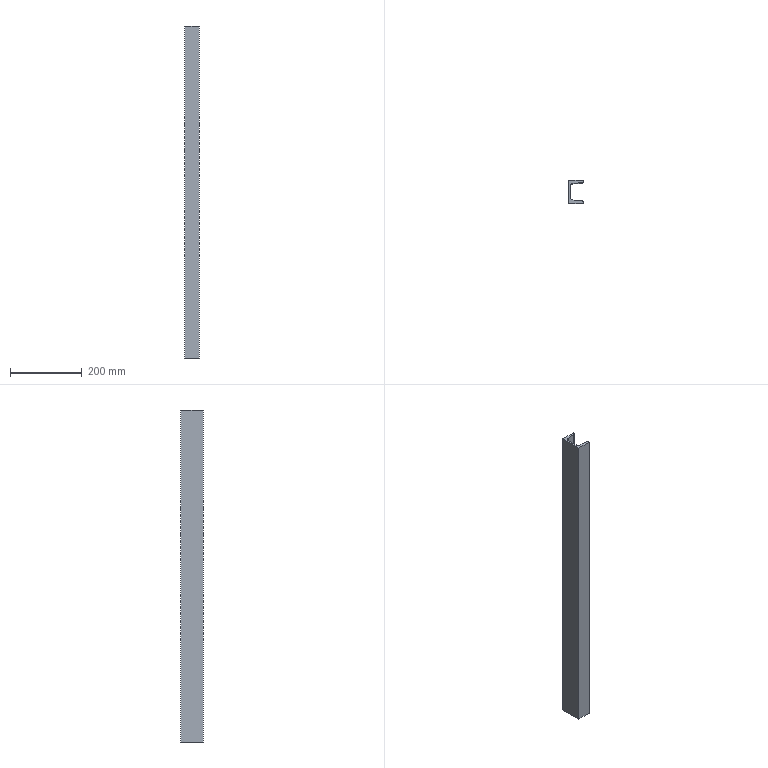Part | STEP file | 750038453 | 1 solid | 14 faces | box 40 x 63 x 924 mm | volume 780380 mm3 | plane 10 | cylinder 4 | commonest cylinder face diameters 7.6 x2 15 x2
STEP:
#1=CARTESIAN_POINT('',(0.,0.,462.));
#2=VERTEX_POINT('',#1);
#3=CARTESIAN_POINT('',(0.,0.,-462.));
#4=VERTEX_POINT('',#3);
#5=CARTESIAN_POINT('',(0.,0.,462.));
#6=DIRECTION('',(0.,0.,-1.));
#7=VECTOR('',#6,1000.);
#8=LINE('',#5,#7);
#9=EDGE_CURVE('',#2,#4,#8,.T.);
#10=ORIENTED_EDGE('',*,*,#9,.F.);
#11=CARTESIAN_POINT('',(0.,63.,462.));
#12=VERTEX_POINT('',#11);
#13=CARTESIAN_POINT('',(0.,63.,462.));
#14=DIRECTION('',(0.,-1.,0.));
#15=VECTOR('',#14,1000.);
#16=LINE('',#13,#15);
#17=EDGE_CURVE('',#12,#2,#16,.T.);
#18=ORIENTED_EDGE('',*,*,#17,.F.);
#19=CARTESIAN_POINT('',(0.,63.,-462.));
#20=VERTEX_POINT('',#19);
#21=CARTESIAN_POINT('',(0.,63.,462.));
#22=DIRECTION('',(0.,0.,1.));
#23=VECTOR('',#22,1000.);
#24=LINE('',#21,#23);
#25=EDGE_CURVE('',#20,#12,#24,.T.);
#26=ORIENTED_EDGE('',*,*,#25,.F.);
#27=CARTESIAN_POINT('',(0.,63.,-462.));
#28=DIRECTION('',(0.,1.,0.));
#29=VECTOR('',#28,1000.);
#30=LINE('',#27,#29);
#31=EDGE_CURVE('',#4,#20,#30,.T.);
#32=ORIENTED_EDGE('',*,*,#31,.F.);
#33=EDGE_LOOP('',(#10,#18,#26,#32));
#34=FACE_OUTER_BOUND('',#33,.T.);
#35=CARTESIAN_POINT('',(0.,63.,462.));
#36=DIRECTION('',(1.,0.,0.));
#37=DIRECTION('',(0.,0.,-1.));
#38=AXIS2_PLACEMENT_3D('',#35,#36,#37);
#39=PLANE('',#38);
#40=ADVANCED_FACE('',(#34),#39,.F.);
#41=CARTESIAN_POINT('',(40.,63.,-462.));
#42=VERTEX_POINT('',#41);
#43=CARTESIAN_POINT('',(36.2,63.,-462.));
#44=DIRECTION('',(-1.,0.,0.));
#45=VECTOR('',#44,1000.);
#46=LINE('',#43,#45);
#47=EDGE_CURVE('',#42,#20,#46,.T.);
#48=ORIENTED_EDGE('',*,*,#47,.F.);
#49=CARTESIAN_POINT('',(40.,60.699,-462.));
#50=VERTEX_POINT('',#49);
#51=CARTESIAN_POINT('',(40.,2.301,-462.));
#52=DIRECTION('',(0.,1.,0.));
#53=VECTOR('',#52,1000.);
#54=LINE('',#51,#53);
#55=EDGE_CURVE('',#50,#42,#54,.T.);
#56=ORIENTED_EDGE('',*,*,#55,.F.);
#57=CARTESIAN_POINT('',(36.578,56.918,-462.));
#58=VERTEX_POINT('',#57);
#59=CARTESIAN_POINT('',(36.2,60.699,-462.));
#60=DIRECTION('',(0.,0.,1.));
#61=DIRECTION('',(-1.,0.,0.));
#62=AXIS2_PLACEMENT_3D('',#59,#60,#61);
#63=CIRCLE('',#62,3.8);
#64=EDGE_CURVE('',#58,#50,#63,.T.);
#65=ORIENTED_EDGE('',*,*,#64,.F.);
#66=CARTESIAN_POINT('',(11.554,54.415,-462.));
#67=VERTEX_POINT('',#66);
#68=CARTESIAN_POINT('',(11.554,54.415,-462.));
#69=DIRECTION('',(0.995,0.0995,0.));
#70=VECTOR('',#69,1000.);
#71=LINE('',#68,#70);
#72=EDGE_CURVE('',#67,#58,#71,.T.);
#73=ORIENTED_EDGE('',*,*,#72,.F.);
#74=CARTESIAN_POINT('',(4.8,46.953,-462.));
#75=VERTEX_POINT('',#74);
#76=CARTESIAN_POINT('',(12.3,46.953,-462.));
#77=DIRECTION('',(0.,0.,-1.));
#78=DIRECTION('',(-1.,0.,0.));
#79=AXIS2_PLACEMENT_3D('',#76,#77,#78);
#80=CIRCLE('',#79,7.5);
#81=EDGE_CURVE('',#75,#67,#80,.T.);
#82=ORIENTED_EDGE('',*,*,#81,.F.);
#83=CARTESIAN_POINT('',(4.8,16.047,-462.));
#84=VERTEX_POINT('',#83);
#85=CARTESIAN_POINT('',(4.8,2.301,-462.));
#86=DIRECTION('',(0.,1.,0.));
#87=VECTOR('',#86,1000.);
#88=LINE('',#85,#87);
#89=EDGE_CURVE('',#84,#75,#88,.T.);
#90=ORIENTED_EDGE('',*,*,#89,.F.);
#91=CARTESIAN_POINT('',(11.554,8.585,-462.));
#92=VERTEX_POINT('',#91);
#93=CARTESIAN_POINT('',(12.3,16.047,-462.));
#94=DIRECTION('',(0.,0.,-1.));
#95=DIRECTION('',(-1.,0.,0.));
#96=AXIS2_PLACEMENT_3D('',#93,#94,#95);
#97=CIRCLE('',#96,7.5);
#98=EDGE_CURVE('',#92,#84,#97,.T.);
#99=ORIENTED_EDGE('',*,*,#98,.F.);
#100=CARTESIAN_POINT('',(36.578,6.082,-462.));
#101=VERTEX_POINT('',#100);
#102=CARTESIAN_POINT('',(36.578,6.082,-462.));
#103=DIRECTION('',(-0.995,0.0995,0.));
#104=VECTOR('',#103,1000.);
#105=LINE('',#102,#104);
#106=EDGE_CURVE('',#101,#92,#105,.T.);
#107=ORIENTED_EDGE('',*,*,#106,.F.);
#108=CARTESIAN_POINT('',(40.,2.301,-462.));
#109=VERTEX_POINT('',#108);
#110=CARTESIAN_POINT('',(36.2,2.301,-462.));
#111=DIRECTION('',(0.,0.,1.));
#112=DIRECTION('',(-1.,0.,0.));
#113=AXIS2_PLACEMENT_3D('',#110,#111,#112);
#114=CIRCLE('',#113,3.8);
#115=EDGE_CURVE('',#109,#101,#114,.T.);
#116=ORIENTED_EDGE('',*,*,#115,.F.);
#117=CARTESIAN_POINT('',(40.,0.,-462.));
#118=VERTEX_POINT('',#117);
#119=CARTESIAN_POINT('',(40.,2.301,-462.));
#120=DIRECTION('',(0.,1.,0.));
#121=VECTOR('',#120,1000.);
#122=LINE('',#119,#121);
#123=EDGE_CURVE('',#118,#109,#122,.T.);
#124=ORIENTED_EDGE('',*,*,#123,.F.);
#125=CARTESIAN_POINT('',(36.2,0.,-462.));
#126=DIRECTION('',(1.,0.,0.));
#127=VECTOR('',#126,1000.);
#128=LINE('',#125,#127);
#129=EDGE_CURVE('',#4,#118,#128,.T.);
#130=ORIENTED_EDGE('',*,*,#129,.F.);
#131=ORIENTED_EDGE('',*,*,#31,.T.);
#132=EDGE_LOOP('',(#48,#56,#65,#73,#82,#90,#99,#107,#116,#124,#130,#131));
#133=FACE_OUTER_BOUND('',#132,.T.);
#134=CARTESIAN_POINT('',(36.2,2.301,-462.));
#135=DIRECTION('',(0.,0.,1.));
#136=DIRECTION('',(1.,0.,0.));
#137=AXIS2_PLACEMENT_3D('',#134,#135,#136);
#138=PLANE('',#137);
#139=ADVANCED_FACE('',(#133),#138,.F.);
#140=CARTESIAN_POINT('',(40.,0.,462.));
#141=VERTEX_POINT('',#140);
#142=CARTESIAN_POINT('',(40.,0.,462.));
#143=DIRECTION('',(0.,0.,-1.));
#144=VECTOR('',#143,1000.);
#145=LINE('',#142,#144);
#146=EDGE_CURVE('',#141,#118,#145,.T.);
#147=ORIENTED_EDGE('',*,*,#146,.F.);
#148=CARTESIAN_POINT('',(0.,0.,462.));
#149=DIRECTION('',(1.,0.,0.));
#150=VECTOR('',#149,1000.);
#151=LINE('',#148,#150);
#152=EDGE_CURVE('',#2,#141,#151,.T.);
#153=ORIENTED_EDGE('',*,*,#152,.F.);
#154=ORIENTED_EDGE('',*,*,#9,.T.);
#155=ORIENTED_EDGE('',*,*,#129,.T.);
#156=EDGE_LOOP('',(#147,#153,#154,#155));
#157=FACE_OUTER_BOUND('',#156,.T.);
#158=CARTESIAN_POINT('',(0.,0.,462.));
#159=DIRECTION('',(0.,1.,0.));
#160=DIRECTION('',(0.,0.,1.));
#161=AXIS2_PLACEMENT_3D('',#158,#159,#160);
#162=PLANE('',#161);
#163=ADVANCED_FACE('',(#157),#162,.F.);
#164=CARTESIAN_POINT('',(40.,60.699,462.));
#165=VERTEX_POINT('',#164);
#166=CARTESIAN_POINT('',(40.,63.,462.));
#167=VERTEX_POINT('',#166);
#168=CARTESIAN_POINT('',(40.,2.301,462.));
#169=DIRECTION('',(0.,1.,0.));
#170=VECTOR('',#169,1000.);
#171=LINE('',#168,#170);
#172=EDGE_CURVE('',#165,#167,#171,.T.);
#173=ORIENTED_EDGE('',*,*,#172,.T.);
#174=CARTESIAN_POINT('',(36.2,63.,462.));
#175=DIRECTION('',(-1.,0.,0.));
#176=VECTOR('',#175,1000.);
#177=LINE('',#174,#176);
#178=EDGE_CURVE('',#167,#12,#177,.T.);
#179=ORIENTED_EDGE('',*,*,#178,.T.);
#180=ORIENTED_EDGE('',*,*,#17,.T.);
#181=ORIENTED_EDGE('',*,*,#152,.T.);
#182=CARTESIAN_POINT('',(40.,2.301,462.));
#183=VERTEX_POINT('',#182);
#184=CARTESIAN_POINT('',(40.,2.301,462.));
#185=DIRECTION('',(0.,1.,0.));
#186=VECTOR('',#185,1000.);
#187=LINE('',#184,#186);
#188=EDGE_CURVE('',#141,#183,#187,.T.);
#189=ORIENTED_EDGE('',*,*,#188,.T.);
#190=CARTESIAN_POINT('',(36.578,6.082,462.));
#191=VERTEX_POINT('',#190);
#192=CARTESIAN_POINT('',(36.2,2.301,462.));
#193=DIRECTION('',(0.,0.,1.));
#194=DIRECTION('',(-1.,0.,0.));
#195=AXIS2_PLACEMENT_3D('',#192,#193,#194);
#196=CIRCLE('',#195,3.8);
#197=EDGE_CURVE('',#183,#191,#196,.T.);
#198=ORIENTED_EDGE('',*,*,#197,.T.);
#199=CARTESIAN_POINT('',(11.554,8.585,462.));
#200=VERTEX_POINT('',#199);
#201=CARTESIAN_POINT('',(36.578,6.082,462.));
#202=DIRECTION('',(-0.995,0.0995,0.));
#203=VECTOR('',#202,1000.);
#204=LINE('',#201,#203);
#205=EDGE_CURVE('',#191,#200,#204,.T.);
#206=ORIENTED_EDGE('',*,*,#205,.T.);
#207=CARTESIAN_POINT('',(4.8,16.047,462.));
#208=VERTEX_POINT('',#207);
#209=CARTESIAN_POINT('',(12.3,16.047,462.));
#210=DIRECTION('',(0.,0.,-1.));
#211=DIRECTION('',(-1.,0.,0.));
#212=AXIS2_PLACEMENT_3D('',#209,#210,#211);
#213=CIRCLE('',#212,7.5);
#214=EDGE_CURVE('',#200,#208,#213,.T.);
#215=ORIENTED_EDGE('',*,*,#214,.T.);
#216=CARTESIAN_POINT('',(4.8,46.953,462.));
#217=VERTEX_POINT('',#216);
#218=CARTESIAN_POINT('',(4.8,2.301,462.));
#219=DIRECTION('',(0.,1.,0.));
#220=VECTOR('',#219,1000.);
#221=LINE('',#218,#220);
#222=EDGE_CURVE('',#208,#217,#221,.T.);
#223=ORIENTED_EDGE('',*,*,#222,.T.);
#224=CARTESIAN_POINT('',(11.554,54.415,462.));
#225=VERTEX_POINT('',#224);
#226=CARTESIAN_POINT('',(12.3,46.953,462.));
#227=DIRECTION('',(0.,0.,-1.));
#228=DIRECTION('',(-1.,0.,0.));
#229=AXIS2_PLACEMENT_3D('',#226,#227,#228);
#230=CIRCLE('',#229,7.5);
#231=EDGE_CURVE('',#217,#225,#230,.T.);
#232=ORIENTED_EDGE('',*,*,#231,.T.);
#233=CARTESIAN_POINT('',(36.578,56.918,462.));
#234=VERTEX_POINT('',#233);
#235=CARTESIAN_POINT('',(11.554,54.415,462.));
#236=DIRECTION('',(0.995,0.0995,0.));
#237=VECTOR('',#236,1000.);
#238=LINE('',#235,#237);
#239=EDGE_CURVE('',#225,#234,#238,.T.);
#240=ORIENTED_EDGE('',*,*,#239,.T.);
#241=CARTESIAN_POINT('',(36.2,60.699,462.));
#242=DIRECTION('',(0.,0.,1.));
#243=DIRECTION('',(-1.,0.,0.));
#244=AXIS2_PLACEMENT_3D('',#241,#242,#243);
#245=CIRCLE('',#244,3.8);
#246=EDGE_CURVE('',#234,#165,#245,.T.);
#247=ORIENTED_EDGE('',*,*,#246,.T.);
#248=EDGE_LOOP('',(#173,#179,#180,#181,#189,#198,#206,#215,#223,#232,#240,#247));
#249=FACE_OUTER_BOUND('',#248,.T.);
#250=CARTESIAN_POINT('',(36.2,2.301,462.));
#251=DIRECTION('',(0.,0.,1.));
#252=DIRECTION('',(1.,0.,0.));
#253=AXIS2_PLACEMENT_3D('',#250,#251,#252);
#254=PLANE('',#253);
#255=ADVANCED_FACE('',(#249),#254,.T.);
#256=ORIENTED_EDGE('',*,*,#25,.T.);
#257=ORIENTED_EDGE('',*,*,#178,.F.);
#258=CARTESIAN_POINT('',(40.,63.,462.));
#259=DIRECTION('',(0.,0.,1.));
#260=VECTOR('',#259,1000.);
#261=LINE('',#258,#260);
#262=EDGE_CURVE('',#42,#167,#261,.T.);
#263=ORIENTED_EDGE('',*,*,#262,.F.);
#264=ORIENTED_EDGE('',*,*,#47,.T.);
#265=EDGE_LOOP('',(#256,#257,#263,#264));
#266=FACE_OUTER_BOUND('',#265,.T.);
#267=CARTESIAN_POINT('',(40.,63.,462.));
#268=DIRECTION('',(0.,-1.,0.));
#269=DIRECTION('',(0.,0.,-1.));
#270=AXIS2_PLACEMENT_3D('',#267,#268,#269);
#271=PLANE('',#270);
#272=ADVANCED_FACE('',(#266),#271,.F.);
#273=ORIENTED_EDGE('',*,*,#262,.T.);
#274=ORIENTED_EDGE('',*,*,#172,.F.);
#275=CARTESIAN_POINT('',(40.,60.699,462.));
#276=DIRECTION('',(0.,0.,1.));
#277=VECTOR('',#276,1000.);
#278=LINE('',#275,#277);
#279=EDGE_CURVE('',#50,#165,#278,.T.);
#280=ORIENTED_EDGE('',*,*,#279,.F.);
#281=ORIENTED_EDGE('',*,*,#55,.T.);
#282=EDGE_LOOP('',(#273,#274,#280,#281));
#283=FACE_OUTER_BOUND('',#282,.T.);
#284=CARTESIAN_POINT('',(40.,60.699,462.));
#285=DIRECTION('',(-1.,0.,0.));
#286=DIRECTION('',(0.,-1.,0.));
#287=AXIS2_PLACEMENT_3D('',#284,#285,#286);
#288=PLANE('',#287);
#289=ADVANCED_FACE('',(#283),#288,.F.);
#290=ORIENTED_EDGE('',*,*,#246,.F.);
#291=CARTESIAN_POINT('',(36.578,56.918,462.));
#292=DIRECTION('',(0.,0.,-1.));
#293=VECTOR('',#292,1000.);
#294=LINE('',#291,#293);
#295=EDGE_CURVE('',#234,#58,#294,.T.);
#296=ORIENTED_EDGE('',*,*,#295,.T.);
#297=ORIENTED_EDGE('',*,*,#64,.T.);
#298=ORIENTED_EDGE('',*,*,#279,.T.);
#299=EDGE_LOOP('',(#290,#296,#297,#298));
#300=FACE_OUTER_BOUND('',#299,.T.);
#301=CARTESIAN_POINT('',(36.2,60.699,462.));
#302=DIRECTION('',(0.,0.,-1.));
#303=DIRECTION('',(-1.,0.,0.));
#304=AXIS2_PLACEMENT_3D('',#301,#302,#303);
#305=CYLINDRICAL_SURFACE('',#304,3.8);
#306=ADVANCED_FACE('',(#300),#305,.T.);
#307=ORIENTED_EDGE('',*,*,#295,.F.);
#308=ORIENTED_EDGE('',*,*,#239,.F.);
#309=CARTESIAN_POINT('',(11.554,54.415,462.));
#310=DIRECTION('',(0.,0.,1.));
#311=VECTOR('',#310,1000.);
#312=LINE('',#309,#311);
#313=EDGE_CURVE('',#67,#225,#312,.T.);
#314=ORIENTED_EDGE('',*,*,#313,.F.);
#315=ORIENTED_EDGE('',*,*,#72,.T.);
#316=EDGE_LOOP('',(#307,#308,#314,#315));
#317=FACE_OUTER_BOUND('',#316,.T.);
#318=CARTESIAN_POINT('',(11.554,54.415,462.));
#319=DIRECTION('',(-0.0995,0.995,0.));
#320=DIRECTION('',(-0.995,-0.0995,0.));
#321=AXIS2_PLACEMENT_3D('',#318,#319,#320);
#322=PLANE('',#321);
#323=ADVANCED_FACE('',(#317),#322,.F.);
#324=ORIENTED_EDGE('',*,*,#313,.T.);
#325=ORIENTED_EDGE('',*,*,#231,.F.);
#326=CARTESIAN_POINT('',(4.8,46.953,462.));
#327=DIRECTION('',(0.,0.,1.));
#328=VECTOR('',#327,1000.);
#329=LINE('',#326,#328);
#330=EDGE_CURVE('',#75,#217,#329,.T.);
#331=ORIENTED_EDGE('',*,*,#330,.F.);
#332=ORIENTED_EDGE('',*,*,#81,.T.);
#333=EDGE_LOOP('',(#324,#325,#331,#332));
#334=FACE_OUTER_BOUND('',#333,.T.);
#335=CARTESIAN_POINT('',(12.3,46.953,462.));
#336=DIRECTION('',(0.,0.,-1.));
#337=DIRECTION('',(-1.,0.,0.));
#338=AXIS2_PLACEMENT_3D('',#335,#336,#337);
#339=CYLINDRICAL_SURFACE('',#338,7.5);
#340=ADVANCED_FACE('',(#334),#339,.F.);
#341=ORIENTED_EDGE('',*,*,#330,.T.);
#342=ORIENTED_EDGE('',*,*,#222,.F.);
#343=CARTESIAN_POINT('',(4.8,16.047,462.));
#344=DIRECTION('',(0.,0.,1.));
#345=VECTOR('',#344,1000.);
#346=LINE('',#343,#345);
#347=EDGE_CURVE('',#84,#208,#346,.T.);
#348=ORIENTED_EDGE('',*,*,#347,.F.);
#349=ORIENTED_EDGE('',*,*,#89,.T.);
#350=EDGE_LOOP('',(#341,#342,#348,#349));
#351=FACE_OUTER_BOUND('',#350,.T.);
#352=CARTESIAN_POINT('',(4.8,16.047,462.));
#353=DIRECTION('',(-1.,0.,0.));
#354=DIRECTION('',(0.,-1.,0.));
#355=AXIS2_PLACEMENT_3D('',#352,#353,#354);
#356=PLANE('',#355);
#357=ADVANCED_FACE('',(#351),#356,.F.);
#358=ORIENTED_EDGE('',*,*,#347,.T.);
#359=ORIENTED_EDGE('',*,*,#214,.F.);
#360=CARTESIAN_POINT('',(11.554,8.585,462.));
#361=DIRECTION('',(0.,0.,1.));
#362=VECTOR('',#361,1000.);
#363=LINE('',#360,#362);
#364=EDGE_CURVE('',#92,#200,#363,.T.);
#365=ORIENTED_EDGE('',*,*,#364,.F.);
#366=ORIENTED_EDGE('',*,*,#98,.T.);
#367=EDGE_LOOP('',(#358,#359,#365,#366));
#368=FACE_OUTER_BOUND('',#367,.T.);
#369=CARTESIAN_POINT('',(12.3,16.047,462.));
#370=DIRECTION('',(0.,0.,-1.));
#371=DIRECTION('',(-1.,0.,0.));
#372=AXIS2_PLACEMENT_3D('',#369,#370,#371);
#373=CYLINDRICAL_SURFACE('',#372,7.5);
#374=ADVANCED_FACE('',(#368),#373,.F.);
#375=ORIENTED_EDGE('',*,*,#364,.T.);
#376=ORIENTED_EDGE('',*,*,#205,.F.);
#377=CARTESIAN_POINT('',(36.578,6.082,462.));
#378=DIRECTION('',(0.,0.,1.));
#379=VECTOR('',#378,1000.);
#380=LINE('',#377,#379);
#381=EDGE_CURVE('',#101,#191,#380,.T.);
#382=ORIENTED_EDGE('',*,*,#381,.F.);
#383=ORIENTED_EDGE('',*,*,#106,.T.);
#384=EDGE_LOOP('',(#375,#376,#382,#383));
#385=FACE_OUTER_BOUND('',#384,.T.);
#386=CARTESIAN_POINT('',(36.578,6.082,462.));
#387=DIRECTION('',(-0.0995,-0.995,0.));
#388=DIRECTION('',(0.995,-0.0995,0.));
#389=AXIS2_PLACEMENT_3D('',#386,#387,#388);
#390=PLANE('',#389);
#391=ADVANCED_FACE('',(#385),#390,.F.);
#392=ORIENTED_EDGE('',*,*,#197,.F.);
#393=CARTESIAN_POINT('',(40.,2.301,462.));
#394=DIRECTION('',(0.,0.,-1.));
#395=VECTOR('',#394,1000.);
#396=LINE('',#393,#395);
#397=EDGE_CURVE('',#183,#109,#396,.T.);
#398=ORIENTED_EDGE('',*,*,#397,.T.);
#399=ORIENTED_EDGE('',*,*,#115,.T.);
#400=ORIENTED_EDGE('',*,*,#381,.T.);
#401=EDGE_LOOP('',(#392,#398,#399,#400));
#402=FACE_OUTER_BOUND('',#401,.T.);
#403=CARTESIAN_POINT('',(36.2,2.301,462.));
#404=DIRECTION('',(0.,0.,-1.));
#405=DIRECTION('',(-1.,0.,0.));
#406=AXIS2_PLACEMENT_3D('',#403,#404,#405);
#407=CYLINDRICAL_SURFACE('',#406,3.8);
#408=ADVANCED_FACE('',(#402),#407,.T.);
#409=ORIENTED_EDGE('',*,*,#397,.F.);
#410=ORIENTED_EDGE('',*,*,#188,.F.);
#411=ORIENTED_EDGE('',*,*,#146,.T.);
#412=ORIENTED_EDGE('',*,*,#123,.T.);
#413=EDGE_LOOP('',(#409,#410,#411,#412));
#414=FACE_OUTER_BOUND('',#413,.T.);
#415=CARTESIAN_POINT('',(40.,0.,462.));
#416=DIRECTION('',(-1.,0.,0.));
#417=DIRECTION('',(0.,0.,1.));
#418=AXIS2_PLACEMENT_3D('',#415,#416,#417);
#419=PLANE('',#418);
#420=ADVANCED_FACE('',(#414),#419,.F.);
#421=CLOSED_SHELL('',(#40,#139,#163,#255,#272,#289,#306,#323,#340,#357,#374,#391,#408,#420));
#422=MANIFOLD_SOLID_BREP('',#421);
#423=CARTESIAN_POINT('',(0.,0.,0.));
#424=DIRECTION('',(0.,0.,1.));
#425=DIRECTION('',(1.,0.,0.));
#426=AXIS2_PLACEMENT_3D('',#423,#424,#425);
#427=(LENGTH_UNIT()NAMED_UNIT(*)SI_UNIT(.MILLI.,.METRE.));
#428=UNCERTAINTY_MEASURE_WITH_UNIT(LENGTH_MEASURE(0.00001),#427,'','');
#429=(NAMED_UNIT(*)PLANE_ANGLE_UNIT()SI_UNIT($,.RADIAN.));
#430=(NAMED_UNIT(*)SI_UNIT($,.STERADIAN.)SOLID_ANGLE_UNIT());
#431=(GEOMETRIC_REPRESENTATION_CONTEXT(3)GLOBAL_UNCERTAINTY_ASSIGNED_CONTEXT((#428))GLOBAL_UNIT_ASSIGNED_CONTEXT((#427,#429,#430))REPRESENTATION_CONTEXT('',''));
#432=ADVANCED_BREP_SHAPE_REPRESENTATION('',(#422,#426),#431);